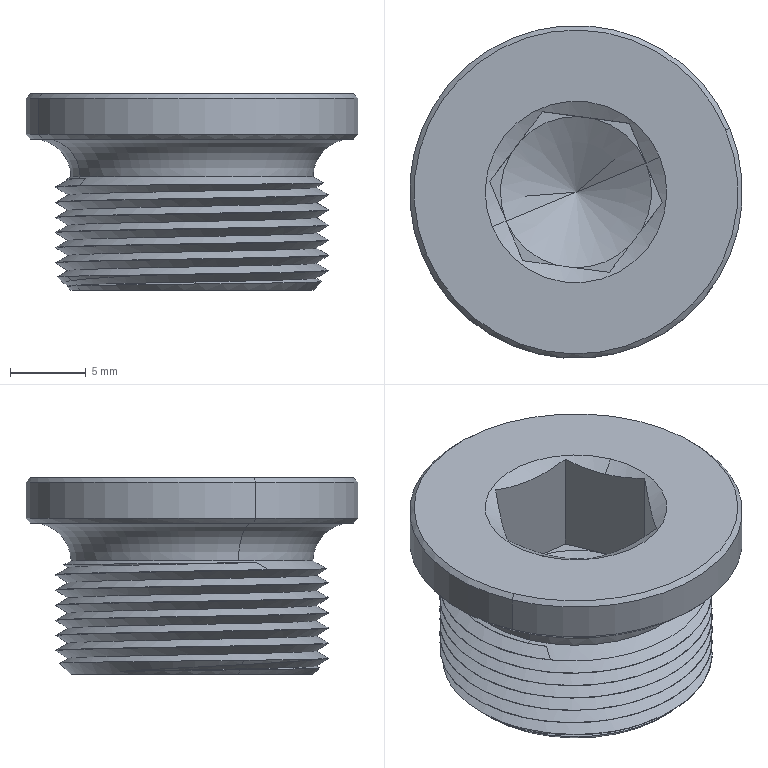Part | SolidWorks | features BaseBody 1 | 1 solid | 51 faces | box 22 x 22 x 13 mm | volume 2755 mm3 | plane 19 | cylinder 15 | cone 13 | torus 2 | spline 2 | commonest cylinder face diameters 18 x13 22 x2